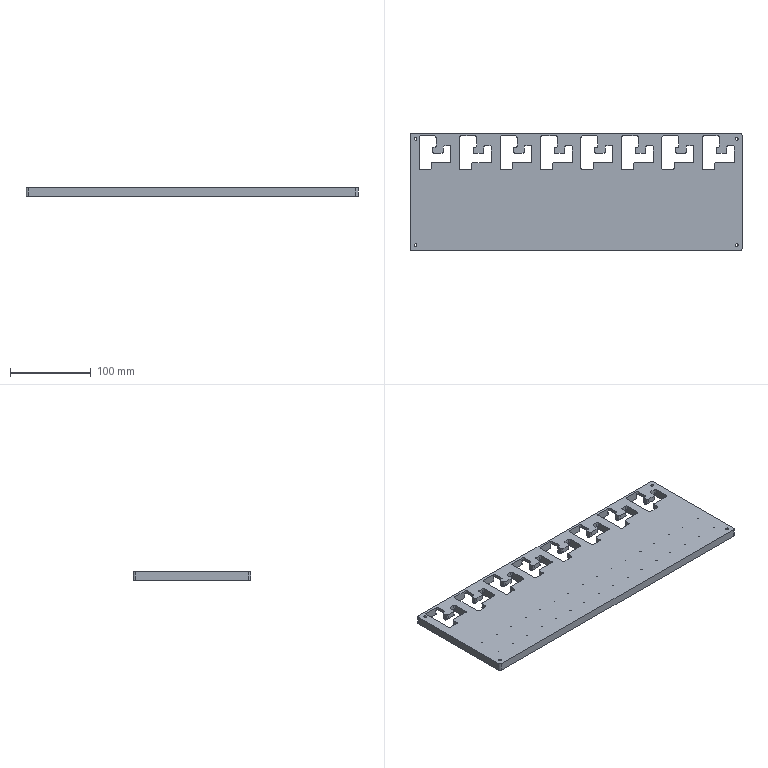NC program | NX | posted with a generic post | part box 410 x 145 x 10 mm
Whole program:
N10 G17 G21 G94 G90
(ZLEVEL_PROFILE_2_COPY_1 , TOOL : D6A45)
N12 T07 M6
N14 G54
N16 G17 G0 G90 X198. Y-66.121 S9500 M3
N18 G43 Z30. H7
N20 Z1.
N22 G94 G1 Z-1. F1250.
N24 G3 X198.621 Y-65.5 R0.621
N26 X198. Y-66.121 R-0.621
N28 X198.52 Y-65.821 R0.6
N30 G1 Z0.
N32 G0 Z30.
N34 X-158.338 Y-49.304
N36 Z0.
N38 G1 Z-1.
N40 X-157.438 Y-48.785
N42 G3 X-157.138 Y-48.265 R0.6
N44 G1 Y-29.041
N46 G3 X-157.908 Y-28.27 R0.771
N48 G1 X-169.295
N50 G3 X-170.066 Y-29.041 R0.771
N52 G1 Y-34.511
N54 G2 X-172.795 Y-37.24 R2.729
N56 G1 X-193.808
N58 G3 X-194.579 Y-38.011 R0.771
N60 G1 Y-55.644
N62 G3 X-193.808 Y-56.415 R0.771
N64 G1 X-188.094
N66 G3 X-187.324 Y-55.644 R0.771
N68 G1 Y-49.623
N70 G2 X-184.594 Y-46.894 R2.729
N72 G1 X-174.741
N74 G2 X-172.012 Y-49.623 R2.729
N76 G1 Y-54.065
N78 G2 X-174.241 Y-56.295 R2.229
N80 G1 X-175.889
N82 G3 X-176.159 Y-56.565 R0.271
N84 G1 Y-67.489
N86 G3 X-175.389 Y-68.26 R0.771
N88 G1 X-157.908
N90 G3 X-157.138 Y-67.489 R0.771
N92 G1 Y-48.265
N94 G3 X-157.438 Y-47.745 R0.6
N96 G1 X-158.338 Y-47.226
N98 Z0.
N100 G0 Z30.
N102 X-108.338 Y-49.304
N104 Z0.
N106 G1 Z-1.
N108 X-107.438 Y-48.785
N110 G3 X-107.138 Y-48.265 R0.6
N112 G1 Y-29.041
N114 G3 X-107.908 Y-28.27 R0.771
N116 G1 X-119.295
N118 G3 X-120.066 Y-29.041 R0.771
N120 G1 Y-34.511
N122 G2 X-122.795 Y-37.24 R2.729
N124 G1 X-143.808
N126 G3 X-144.579 Y-38.011 R0.771
N128 G1 Y-55.644
N130 G3 X-143.808 Y-56.415 R0.771
N132 G1 X-138.094
N134 G3 X-137.324 Y-55.644 R0.771
N136 G1 Y-49.623
N138 G2 X-134.594 Y-46.894 R2.729
N140 G1 X-124.741
N142 G2 X-122.012 Y-49.623 R2.729
N144 G1 Y-54.065
N146 G2 X-124.241 Y-56.295 R2.229
N148 G1 X-125.889
N150 G3 X-126.159 Y-56.565 R0.271
N152 G1 Y-67.489
N154 G3 X-125.389 Y-68.26 R0.771
N156 G1 X-107.908
N158 G3 X-107.138 Y-67.489 R0.771
N160 G1 Y-48.265
N162 G3 X-107.438 Y-47.745 R0.6
N164 G1 X-108.338 Y-47.226
N166 Z0.
N168 G0 Z30.
N170 X-58.338 Y-49.304
N172 Z0.
N174 G1 Z-1.
N176 X-57.438 Y-48.785
N178 G3 X-57.138 Y-48.265 R0.6
N180 G1 Y-29.041
N182 G3 X-57.908 Y-28.27 R0.771
N184 G1 X-69.295
N186 G3 X-70.066 Y-29.041 R0.771
N188 G1 Y-34.511
N190 G2 X-72.795 Y-37.24 R2.729
N192 G1 X-93.808
N194 G3 X-94.579 Y-38.011 R0.771
N196 G1 Y-55.644
N198 G3 X-93.808 Y-56.415 R0.771
N200 G1 X-88.094
N202 G3 X-87.324 Y-55.644 R0.771
N204 G1 Y-49.623
N206 G2 X-84.594 Y-46.894 R2.729
N208 G1 X-74.741
N210 G2 X-72.012 Y-49.623 R2.729
N212 G1 Y-54.065
N214 G2 X-74.241 Y-56.295 R2.229
N216 G1 X-75.889
N218 G3 X-76.159 Y-56.565 R0.271
N220 G1 Y-67.489
N222 G3 X-75.389 Y-68.26 R0.771
N224 G1 X-57.908
N226 G3 X-57.138 Y-67.489 R0.771
N228 G1 Y-48.265
N230 G3 X-57.438 Y-47.745 R0.6
N232 G1 X-58.338 Y-47.226
N234 Z0.
N236 G0 Z30.
N238 X-8.338 Y-49.304
N240 Z0.
N242 G1 Z-1.
N244 X-7.438 Y-48.785
N246 G3 X-7.138 Y-48.265 R0.6
N248 G1 Y-29.041
N250 G3 X-7.908 Y-28.27 R0.771
N252 G1 X-19.295
N254 G3 X-20.066 Y-29.041 R0.771
N256 G1 Y-34.511
N258 G2 X-22.795 Y-37.24 R2.729
N260 G1 X-43.808
N262 G3 X-44.579 Y-38.011 R0.771
N264 G1 Y-55.644
N266 G3 X-43.808 Y-56.415 R0.771
N268 G1 X-38.094
N270 G3 X-37.324 Y-55.644 R0.771
N272 G1 Y-49.623
N274 G2 X-34.594 Y-46.894 R2.729
N276 G1 X-24.741
N278 G2 X-22.012 Y-49.623 R2.729
N280 G1 Y-54.065
N282 G2 X-24.241 Y-56.295 R2.229
N284 G1 X-25.889
N286 G3 X-26.159 Y-56.565 R0.271
N288 G1 Y-67.489
N290 G3 X-25.389 Y-68.26 R0.771
N292 G1 X-7.908
N294 G3 X-7.138 Y-67.489 R0.771
N296 G1 Y-48.265
N298 G3 X-7.438 Y-47.745 R0.6
N300 G1 X-8.338 Y-47.226
N302 Z0.
N304 G0 Z30.
N306 X41.662 Y-49.304
N308 Z0.
N310 G1 Z-1.
N312 X42.562 Y-48.785
N314 G3 X42.862 Y-48.265 R0.6
N316 G1 Y-29.041
N318 G3 X42.092 Y-28.27 R0.771
N320 G1 X30.705
N322 G3 X29.934 Y-29.041 R0.771
N324 G1 Y-34.511
N326 G2 X27.205 Y-37.24 R2.729
N328 G1 X6.192
N330 G3 X5.421 Y-38.011 R0.771
N332 G1 Y-55.644
N334 G3 X6.192 Y-56.415 R0.771
N336 G1 X11.906
N338 G3 X12.676 Y-55.644 R0.771
N340 G1 Y-49.623
N342 G2 X15.406 Y-46.894 R2.729
N344 G1 X25.259
N346 G2 X27.988 Y-49.623 R2.729
N348 G1 Y-54.065
N350 G2 X25.759 Y-56.295 R2.229
N352 G1 X24.111
N354 G3 X23.841 Y-56.565 R0.271
N356 G1 Y-67.489
N358 G3 X24.611 Y-68.26 R0.771
N360 G1 X42.092
N362 G3 X42.862 Y-67.489 R0.771
N364 G1 Y-48.265
N366 G3 X42.562 Y-47.745 R0.6
N368 G1 X41.662 Y-47.226
N370 Z0.
N372 G0 Z30.
N374 X91.662 Y-49.304
N376 Z0.
N378 G1 Z-1.
N380 X92.562 Y-48.785
N382 G3 X92.862 Y-48.265 R0.6
N384 G1 Y-29.041
N386 G3 X92.092 Y-28.27 R0.771
N388 G1 X80.705
N390 G3 X79.934 Y-29.041 R0.771
N392 G1 Y-34.511
N394 G2 X77.205 Y-37.24 R2.729
N396 G1 X56.192
N398 G3 X55.421 Y-38.011 R0.771
N400 G1 Y-55.644
N402 G3 X56.192 Y-56.415 R0.771
N404 G1 X61.906
N406 G3 X62.676 Y-55.644 R0.771
N408 G1 Y-49.623
N410 G2 X65.406 Y-46.894 R2.729
N412 G1 X75.259
N414 G2 X77.988 Y-49.623 R2.729
N416 G1 Y-54.065
N418 G2 X75.759 Y-56.295 R2.229
N420 G1 X74.111
N422 G3 X73.841 Y-56.565 R0.271
N424 G1 Y-67.489
N426 G3 X74.611 Y-68.26 R0.771
N428 G1 X92.092
N430 G3 X92.862 Y-67.489 R0.771
N432 G1 Y-48.265
N434 G3 X92.562 Y-47.745 R0.6
N436 G1 X91.662 Y-47.226
N438 Z0.
N440 G0 Z30.
N442 X141.662 Y-49.304
N444 Z0.
N446 G1 Z-1.
N448 X142.562 Y-48.785
N450 G3 X142.862 Y-48.265 R0.6
N452 G1 Y-29.041
N454 G3 X142.092 Y-28.27 R0.771
N456 G1 X130.705
N458 G3 X129.934 Y-29.041 R0.771
N460 G1 Y-34.511
N462 G2 X127.205 Y-37.24 R2.729
N464 G1 X106.192
N466 G3 X105.421 Y-38.011 R0.771
N468 G1 Y-55.644
N470 G3 X106.192 Y-56.415 R0.771
N472 G1 X111.906
N474 G3 X112.676 Y-55.644 R0.771
N476 G1 Y-49.623
N478 G2 X115.406 Y-46.894 R2.729
N480 G1 X125.259
N482 G2 X127.988 Y-49.623 R2.729
N484 G1 Y-54.065
N486 G2 X125.759 Y-56.295 R2.229
N488 G1 X124.111
N490 G3 X123.841 Y-56.565 R0.271
N492 G1 Y-67.489
N494 G3 X124.611 Y-68.26 R0.771
N496 G1 X142.092
N498 G3 X142.862 Y-67.489 R0.771
N500 G1 Y-48.265
N502 G3 X142.562 Y-47.745 R0.6
N504 G1 X141.662 Y-47.226
N506 Z0.
N508 G0 Z30.
N510 X191.662 Y-49.304
N512 Z0.
N514 G1 Z-1.
N516 X192.562 Y-48.785
N518 G3 X192.862 Y-48.265 R0.6
N520 G1 Y-29.041
N522 G3 X192.092 Y-28.27 R0.771
N524 G1 X180.705
N526 G3 X179.934 Y-29.041 R0.771
N528 G1 Y-34.511
N530 G2 X177.205 Y-37.24 R2.729
N532 G1 X156.192
N534 G3 X155.421 Y-38.011 R0.771
N536 G1 Y-55.644
N538 G3 X156.192 Y-56.415 R0.771
N540 G1 X161.906
N542 G3 X162.676 Y-55.644 R0.771
N544 G1 Y-49.623
N546 G2 X165.406 Y-46.894 R2.729
N548 G1 X175.259
N550 G2 X177.988 Y-49.623 R2.729
N552 G1 Y-54.065
N554 G2 X175.759 Y-56.295 R2.229
N556 G1 X174.111
N558 G3 X173.841 Y-56.565 R0.271
N560 G1 Y-67.489
N562 G3 X174.611 Y-68.26 R0.771
N564 G1 X192.092
N566 G3 X192.862 Y-67.489 R0.771
N568 G1 Y-48.265
N570 G3 X192.562 Y-47.745 R0.6
N572 G1 X191.662 Y-47.226
N574 Z0.
N576 G0 Z30.
N578 X-199.121 Y65.5
N580 Z1.
N582 G1 Z-1.
N584 G3 X-198.5 Y64.879 R0.621
N586 X-199.121 Y65.5 R-0.621
N588 X-198.821 Y64.98 R0.6
N590 G1 Z0.
N592 G0 Z30.
N594 X198. Y66.121
N596 Z1.
N598 G1 Z-1.
N600 X197.983 Y66.12
N602 G3 X198. Y66.121 R-0.621
N604 X197.48 Y65.821 R0.6
N606 G1 Z0.
N608 G0 Z30.
N610 X-199.121 Y-65.5
N612 Z1.
N614 G1 Z-1.
N616 G3 X-198.5 Y-66.121 R0.621
N618 X-199.121 Y-65.5 R-0.621
N620 X-198.821 Y-66.02 R0.6
N622 G1 Z0.
N624 G0 Z30.
N626 X1.039 Y-74.679
N628 Z0.
N630 G1 Z-1.
N632 X0.52 Y-73.779
N634 G3 X0. Y-73.479 R0.6
N636 G1 X-202.5
N638 G2 X-205.979 Y-70. R3.479
N640 G1 Y70.
N642 G2 X-202.5 Y73.479 R3.479
N644 G1 X202.5
N646 G2 X205.979 Y70. R3.479
N648 G1 Y-70.
N650 G2 X202.5 Y-73.479 R3.479
N652 G1 X0.
N654 G3 X-0.52 Y-73.779 R0.6
N656 G1 X-1.039 Y-74.679
N658 Z0.
N660 G0 Z30.
N662 M5
N664 M2